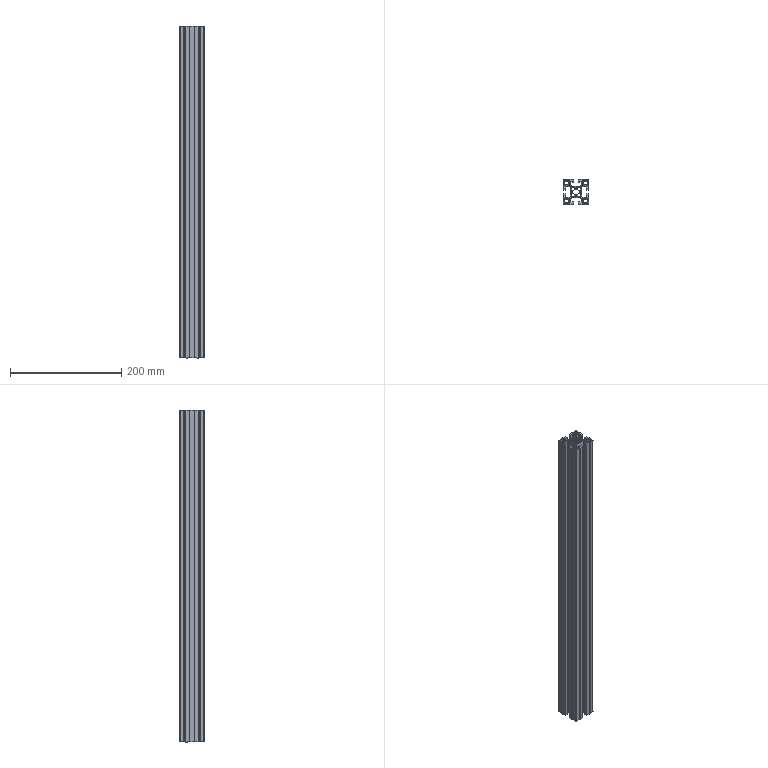Part | STEP file | 4545-765 aluminium profile (upper short) | 1 solid | 262 faces | box 45 x 45 x 597.5 mm | volume 414574 mm3 | plane 186 | cylinder 76 | commonest cylinder face diameters 2 x44 8 x20 12 x8 4 x4